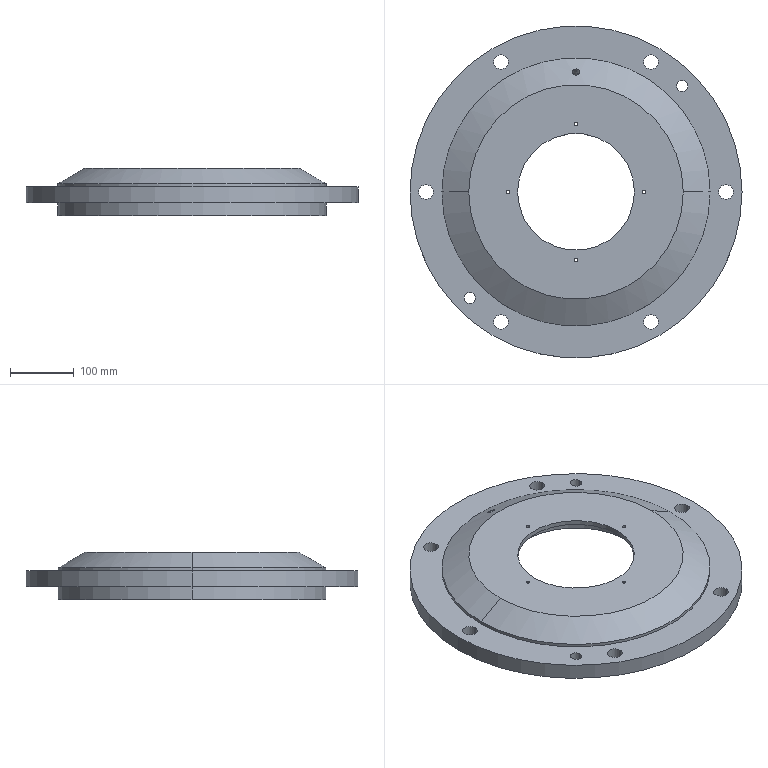Part | SolidWorks | features MirrorStock 1 | 1 solid | 51 faces | box 520 x 520 x 74 mm | volume 4938008 mm3 | cylinder 38 | plane 7 | cone 4 | torus 2 | commonest cylinder face diameters 23 x12 5 x8 17.5 x4 420 x4 10.7 x2 183 x2